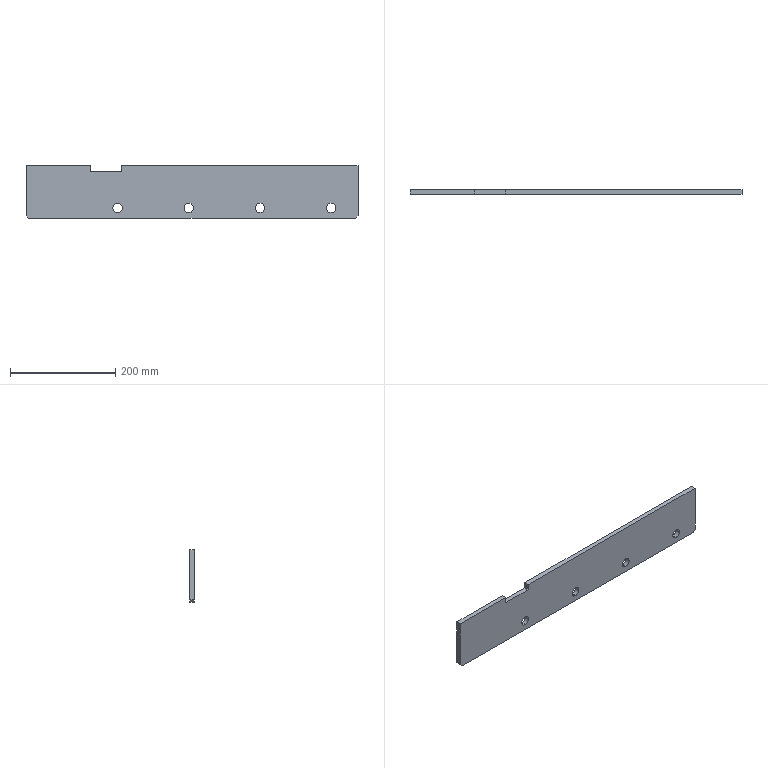Part | SolidWorks | features FlatPattern 1, SMBaseFlange 1, SheetMetal 1 | 1 solid | 20 faces | box 630 x 9 x 100 mm | volume 551134 mm3 | plane 12 | cylinder 8 | commonest cylinder face diameters 18 x8
STEP:
#1=CARTESIAN_POINT('',(579.,-9.,-89.));
#2=VERTEX_POINT('',#1);
#3=CARTESIAN_POINT('',(579.,-9.,-71.));
#4=VERTEX_POINT('',#3);
#5=CARTESIAN_POINT('',(579.,-9.,-80.));
#6=DIRECTION('',(0.,1.,0.));
#7=DIRECTION('',(0.,0.,1.));
#8=AXIS2_PLACEMENT_3D('',#5,#6,#7);
#9=CIRCLE('',#8,9.);
#10=EDGE_CURVE('',#2,#4,#9,.T.);
#11=ORIENTED_EDGE('',*,*,#10,.F.);
#12=CARTESIAN_POINT('',(579.,0.,-89.));
#13=VERTEX_POINT('',#12);
#14=CARTESIAN_POINT('',(579.,-9.,-89.));
#15=DIRECTION('',(0.,1.,0.));
#16=VECTOR('',#15,1000.);
#17=LINE('',#14,#16);
#18=EDGE_CURVE('',#2,#13,#17,.T.);
#19=ORIENTED_EDGE('',*,*,#18,.T.);
#20=CARTESIAN_POINT('',(579.,0.,-71.));
#21=VERTEX_POINT('',#20);
#22=CARTESIAN_POINT('',(579.,0.,-80.));
#23=DIRECTION('',(0.,1.,0.));
#24=DIRECTION('',(0.,0.,1.));
#25=AXIS2_PLACEMENT_3D('',#22,#23,#24);
#26=CIRCLE('',#25,9.);
#27=EDGE_CURVE('',#13,#21,#26,.T.);
#28=ORIENTED_EDGE('',*,*,#27,.T.);
#29=CARTESIAN_POINT('',(579.,-9.,-71.));
#30=DIRECTION('',(0.,1.,0.));
#31=VECTOR('',#30,1000.);
#32=LINE('',#29,#31);
#33=EDGE_CURVE('',#4,#21,#32,.T.);
#34=ORIENTED_EDGE('',*,*,#33,.F.);
#35=EDGE_LOOP('',(#11,#19,#28,#34));
#36=FACE_OUTER_BOUND('',#35,.T.);
#37=CARTESIAN_POINT('',(579.,-9.,-80.));
#38=DIRECTION('',(0.,1.,0.));
#39=DIRECTION('',(0.,0.,1.));
#40=AXIS2_PLACEMENT_3D('',#37,#38,#39);
#41=CYLINDRICAL_SURFACE('',#40,9.);
#42=ADVANCED_FACE('',(#36),#41,.F.);
#43=CARTESIAN_POINT('',(444.,-9.,-89.));
#44=VERTEX_POINT('',#43);
#45=CARTESIAN_POINT('',(444.,-9.,-71.));
#46=VERTEX_POINT('',#45);
#47=CARTESIAN_POINT('',(444.,-9.,-80.));
#48=DIRECTION('',(0.,1.,0.));
#49=DIRECTION('',(0.,0.,1.));
#50=AXIS2_PLACEMENT_3D('',#47,#48,#49);
#51=CIRCLE('',#50,9.);
#52=EDGE_CURVE('',#44,#46,#51,.T.);
#53=ORIENTED_EDGE('',*,*,#52,.F.);
#54=CARTESIAN_POINT('',(444.,0.,-89.));
#55=VERTEX_POINT('',#54);
#56=CARTESIAN_POINT('',(444.,-9.,-89.));
#57=DIRECTION('',(0.,1.,0.));
#58=VECTOR('',#57,1000.);
#59=LINE('',#56,#58);
#60=EDGE_CURVE('',#44,#55,#59,.T.);
#61=ORIENTED_EDGE('',*,*,#60,.T.);
#62=CARTESIAN_POINT('',(444.,0.,-71.));
#63=VERTEX_POINT('',#62);
#64=CARTESIAN_POINT('',(444.,0.,-80.));
#65=DIRECTION('',(0.,1.,0.));
#66=DIRECTION('',(0.,0.,1.));
#67=AXIS2_PLACEMENT_3D('',#64,#65,#66);
#68=CIRCLE('',#67,9.);
#69=EDGE_CURVE('',#55,#63,#68,.T.);
#70=ORIENTED_EDGE('',*,*,#69,.T.);
#71=CARTESIAN_POINT('',(444.,-9.,-71.));
#72=DIRECTION('',(0.,1.,0.));
#73=VECTOR('',#72,1000.);
#74=LINE('',#71,#73);
#75=EDGE_CURVE('',#46,#63,#74,.T.);
#76=ORIENTED_EDGE('',*,*,#75,.F.);
#77=EDGE_LOOP('',(#53,#61,#70,#76));
#78=FACE_OUTER_BOUND('',#77,.T.);
#79=CARTESIAN_POINT('',(444.,-9.,-80.));
#80=DIRECTION('',(0.,1.,0.));
#81=DIRECTION('',(0.,0.,1.));
#82=AXIS2_PLACEMENT_3D('',#79,#80,#81);
#83=CYLINDRICAL_SURFACE('',#82,9.);
#84=ADVANCED_FACE('',(#78),#83,.F.);
#85=CARTESIAN_POINT('',(309.,-9.,-89.));
#86=VERTEX_POINT('',#85);
#87=CARTESIAN_POINT('',(309.,-9.,-71.));
#88=VERTEX_POINT('',#87);
#89=CARTESIAN_POINT('',(309.,-9.,-80.));
#90=DIRECTION('',(0.,1.,0.));
#91=DIRECTION('',(0.,0.,1.));
#92=AXIS2_PLACEMENT_3D('',#89,#90,#91);
#93=CIRCLE('',#92,9.);
#94=EDGE_CURVE('',#86,#88,#93,.T.);
#95=ORIENTED_EDGE('',*,*,#94,.F.);
#96=CARTESIAN_POINT('',(309.,0.,-89.));
#97=VERTEX_POINT('',#96);
#98=CARTESIAN_POINT('',(309.,-9.,-89.));
#99=DIRECTION('',(0.,1.,0.));
#100=VECTOR('',#99,1000.);
#101=LINE('',#98,#100);
#102=EDGE_CURVE('',#86,#97,#101,.T.);
#103=ORIENTED_EDGE('',*,*,#102,.T.);
#104=CARTESIAN_POINT('',(309.,0.,-71.));
#105=VERTEX_POINT('',#104);
#106=CARTESIAN_POINT('',(309.,0.,-80.));
#107=DIRECTION('',(0.,1.,0.));
#108=DIRECTION('',(0.,0.,1.));
#109=AXIS2_PLACEMENT_3D('',#106,#107,#108);
#110=CIRCLE('',#109,9.);
#111=EDGE_CURVE('',#97,#105,#110,.T.);
#112=ORIENTED_EDGE('',*,*,#111,.T.);
#113=CARTESIAN_POINT('',(309.,-9.,-71.));
#114=DIRECTION('',(0.,1.,0.));
#115=VECTOR('',#114,1000.);
#116=LINE('',#113,#115);
#117=EDGE_CURVE('',#88,#105,#116,.T.);
#118=ORIENTED_EDGE('',*,*,#117,.F.);
#119=EDGE_LOOP('',(#95,#103,#112,#118));
#120=FACE_OUTER_BOUND('',#119,.T.);
#121=CARTESIAN_POINT('',(309.,-9.,-80.));
#122=DIRECTION('',(0.,1.,0.));
#123=DIRECTION('',(0.,0.,1.));
#124=AXIS2_PLACEMENT_3D('',#121,#122,#123);
#125=CYLINDRICAL_SURFACE('',#124,9.);
#126=ADVANCED_FACE('',(#120),#125,.F.);
#127=CARTESIAN_POINT('',(174.,-9.,-89.));
#128=VERTEX_POINT('',#127);
#129=CARTESIAN_POINT('',(174.,-9.,-71.));
#130=VERTEX_POINT('',#129);
#131=CARTESIAN_POINT('',(174.,-9.,-80.));
#132=DIRECTION('',(0.,1.,0.));
#133=DIRECTION('',(0.,0.,1.));
#134=AXIS2_PLACEMENT_3D('',#131,#132,#133);
#135=CIRCLE('',#134,9.);
#136=EDGE_CURVE('',#128,#130,#135,.T.);
#137=ORIENTED_EDGE('',*,*,#136,.F.);
#138=CARTESIAN_POINT('',(174.,0.,-89.));
#139=VERTEX_POINT('',#138);
#140=CARTESIAN_POINT('',(174.,-9.,-89.));
#141=DIRECTION('',(0.,1.,0.));
#142=VECTOR('',#141,1000.);
#143=LINE('',#140,#142);
#144=EDGE_CURVE('',#128,#139,#143,.T.);
#145=ORIENTED_EDGE('',*,*,#144,.T.);
#146=CARTESIAN_POINT('',(174.,0.,-71.));
#147=VERTEX_POINT('',#146);
#148=CARTESIAN_POINT('',(174.,0.,-80.));
#149=DIRECTION('',(0.,1.,0.));
#150=DIRECTION('',(0.,0.,1.));
#151=AXIS2_PLACEMENT_3D('',#148,#149,#150);
#152=CIRCLE('',#151,9.);
#153=EDGE_CURVE('',#139,#147,#152,.T.);
#154=ORIENTED_EDGE('',*,*,#153,.T.);
#155=CARTESIAN_POINT('',(174.,-9.,-71.));
#156=DIRECTION('',(0.,1.,0.));
#157=VECTOR('',#156,1000.);
#158=LINE('',#155,#157);
#159=EDGE_CURVE('',#130,#147,#158,.T.);
#160=ORIENTED_EDGE('',*,*,#159,.F.);
#161=EDGE_LOOP('',(#137,#145,#154,#160));
#162=FACE_OUTER_BOUND('',#161,.T.);
#163=CARTESIAN_POINT('',(174.,-9.,-80.));
#164=DIRECTION('',(0.,1.,0.));
#165=DIRECTION('',(0.,0.,1.));
#166=AXIS2_PLACEMENT_3D('',#163,#164,#165);
#167=CYLINDRICAL_SURFACE('',#166,9.);
#168=ADVANCED_FACE('',(#162),#167,.F.);
#169=CARTESIAN_POINT('',(0.,0.,-95.));
#170=VERTEX_POINT('',#169);
#171=CARTESIAN_POINT('',(0.,0.,0.));
#172=VERTEX_POINT('',#171);
#173=CARTESIAN_POINT('',(0.,0.,0.));
#174=DIRECTION('',(0.,0.,1.));
#175=VECTOR('',#174,1000.);
#176=LINE('',#173,#175);
#177=EDGE_CURVE('',#170,#172,#176,.T.);
#178=ORIENTED_EDGE('',*,*,#177,.F.);
#179=CARTESIAN_POINT('',(0.,-9.,-95.));
#180=VERTEX_POINT('',#179);
#181=CARTESIAN_POINT('',(0.,-9.,-95.));
#182=DIRECTION('',(0.,1.,0.));
#183=VECTOR('',#182,1000.);
#184=LINE('',#181,#183);
#185=EDGE_CURVE('',#180,#170,#184,.T.);
#186=ORIENTED_EDGE('',*,*,#185,.F.);
#187=CARTESIAN_POINT('',(0.,-9.,0.));
#188=VERTEX_POINT('',#187);
#189=CARTESIAN_POINT('',(0.,-9.,0.));
#190=DIRECTION('',(0.,0.,1.));
#191=VECTOR('',#190,1000.);
#192=LINE('',#189,#191);
#193=EDGE_CURVE('',#180,#188,#192,.T.);
#194=ORIENTED_EDGE('',*,*,#193,.T.);
#195=CARTESIAN_POINT('',(0.,-9.,0.));
#196=DIRECTION('',(0.,1.,0.));
#197=VECTOR('',#196,1000.);
#198=LINE('',#195,#197);
#199=EDGE_CURVE('',#188,#172,#198,.T.);
#200=ORIENTED_EDGE('',*,*,#199,.T.);
#201=EDGE_LOOP('',(#178,#186,#194,#200));
#202=FACE_OUTER_BOUND('',#201,.T.);
#203=CARTESIAN_POINT('',(0.,-9.,0.));
#204=DIRECTION('',(-1.,0.,0.));
#205=DIRECTION('',(0.,0.,1.));
#206=AXIS2_PLACEMENT_3D('',#203,#204,#205);
#207=PLANE('',#206);
#208=ADVANCED_FACE('',(#202),#207,.T.);
#209=CARTESIAN_POINT('',(5.,0.,-100.));
#210=VERTEX_POINT('',#209);
#211=CARTESIAN_POINT('',(0.,0.,-95.));
#212=DIRECTION('',(-0.7071,0.,0.7071));
#213=VECTOR('',#212,1000.);
#214=LINE('',#211,#213);
#215=EDGE_CURVE('',#210,#170,#214,.T.);
#216=ORIENTED_EDGE('',*,*,#215,.F.);
#217=CARTESIAN_POINT('',(5.,-9.,-100.));
#218=VERTEX_POINT('',#217);
#219=CARTESIAN_POINT('',(5.,-9.,-100.));
#220=DIRECTION('',(0.,1.,0.));
#221=VECTOR('',#220,1000.);
#222=LINE('',#219,#221);
#223=EDGE_CURVE('',#218,#210,#222,.T.);
#224=ORIENTED_EDGE('',*,*,#223,.F.);
#225=CARTESIAN_POINT('',(0.,-9.,-95.));
#226=DIRECTION('',(-0.7071,0.,0.7071));
#227=VECTOR('',#226,1000.);
#228=LINE('',#225,#227);
#229=EDGE_CURVE('',#218,#180,#228,.T.);
#230=ORIENTED_EDGE('',*,*,#229,.T.);
#231=ORIENTED_EDGE('',*,*,#185,.T.);
#232=EDGE_LOOP('',(#216,#224,#230,#231));
#233=FACE_OUTER_BOUND('',#232,.T.);
#234=CARTESIAN_POINT('',(0.,-9.,-95.));
#235=DIRECTION('',(-0.7071,0.,-0.7071));
#236=DIRECTION('',(-0.7071,0.,0.7071));
#237=AXIS2_PLACEMENT_3D('',#234,#235,#236);
#238=PLANE('',#237);
#239=ADVANCED_FACE('',(#233),#238,.T.);
#240=CARTESIAN_POINT('',(625.,0.,-100.));
#241=VERTEX_POINT('',#240);
#242=CARTESIAN_POINT('',(5.,0.,-100.));
#243=DIRECTION('',(-1.,0.,0.));
#244=VECTOR('',#243,1000.);
#245=LINE('',#242,#244);
#246=EDGE_CURVE('',#241,#210,#245,.T.);
#247=ORIENTED_EDGE('',*,*,#246,.F.);
#248=CARTESIAN_POINT('',(625.,-9.,-100.));
#249=VERTEX_POINT('',#248);
#250=CARTESIAN_POINT('',(625.,-9.,-100.));
#251=DIRECTION('',(0.,1.,0.));
#252=VECTOR('',#251,1000.);
#253=LINE('',#250,#252);
#254=EDGE_CURVE('',#249,#241,#253,.T.);
#255=ORIENTED_EDGE('',*,*,#254,.F.);
#256=CARTESIAN_POINT('',(5.,-9.,-100.));
#257=DIRECTION('',(-1.,0.,0.));
#258=VECTOR('',#257,1000.);
#259=LINE('',#256,#258);
#260=EDGE_CURVE('',#249,#218,#259,.T.);
#261=ORIENTED_EDGE('',*,*,#260,.T.);
#262=ORIENTED_EDGE('',*,*,#223,.T.);
#263=EDGE_LOOP('',(#247,#255,#261,#262));
#264=FACE_OUTER_BOUND('',#263,.T.);
#265=CARTESIAN_POINT('',(5.,-9.,-100.));
#266=DIRECTION('',(0.,0.,-1.));
#267=DIRECTION('',(-1.,0.,0.));
#268=AXIS2_PLACEMENT_3D('',#265,#266,#267);
#269=PLANE('',#268);
#270=ADVANCED_FACE('',(#264),#269,.T.);
#271=CARTESIAN_POINT('',(630.,0.,-95.));
#272=VERTEX_POINT('',#271);
#273=CARTESIAN_POINT('',(625.,0.,-100.));
#274=DIRECTION('',(-0.7071,0.,-0.7071));
#275=VECTOR('',#274,1000.);
#276=LINE('',#273,#275);
#277=EDGE_CURVE('',#272,#241,#276,.T.);
#278=ORIENTED_EDGE('',*,*,#277,.F.);
#279=CARTESIAN_POINT('',(630.,-9.,-95.));
#280=VERTEX_POINT('',#279);
#281=CARTESIAN_POINT('',(630.,-9.,-95.));
#282=DIRECTION('',(0.,1.,0.));
#283=VECTOR('',#282,1000.);
#284=LINE('',#281,#283);
#285=EDGE_CURVE('',#280,#272,#284,.T.);
#286=ORIENTED_EDGE('',*,*,#285,.F.);
#287=CARTESIAN_POINT('',(625.,-9.,-100.));
#288=DIRECTION('',(-0.7071,0.,-0.7071));
#289=VECTOR('',#288,1000.);
#290=LINE('',#287,#289);
#291=EDGE_CURVE('',#280,#249,#290,.T.);
#292=ORIENTED_EDGE('',*,*,#291,.T.);
#293=ORIENTED_EDGE('',*,*,#254,.T.);
#294=EDGE_LOOP('',(#278,#286,#292,#293));
#295=FACE_OUTER_BOUND('',#294,.T.);
#296=CARTESIAN_POINT('',(625.,-9.,-100.));
#297=DIRECTION('',(0.7071,0.,-0.7071));
#298=DIRECTION('',(-0.7071,0.,-0.7071));
#299=AXIS2_PLACEMENT_3D('',#296,#297,#298);
#300=PLANE('',#299);
#301=ADVANCED_FACE('',(#295),#300,.T.);
#302=CARTESIAN_POINT('',(630.,0.,0.));
#303=VERTEX_POINT('',#302);
#304=CARTESIAN_POINT('',(630.,0.,0.));
#305=DIRECTION('',(0.,0.,-1.));
#306=VECTOR('',#305,1000.);
#307=LINE('',#304,#306);
#308=EDGE_CURVE('',#303,#272,#307,.T.);
#309=ORIENTED_EDGE('',*,*,#308,.F.);
#310=CARTESIAN_POINT('',(630.,-9.,0.));
#311=VERTEX_POINT('',#310);
#312=CARTESIAN_POINT('',(630.,-9.,0.));
#313=DIRECTION('',(0.,1.,0.));
#314=VECTOR('',#313,1000.);
#315=LINE('',#312,#314);
#316=EDGE_CURVE('',#311,#303,#315,.T.);
#317=ORIENTED_EDGE('',*,*,#316,.F.);
#318=CARTESIAN_POINT('',(630.,-9.,0.));
#319=DIRECTION('',(0.,0.,-1.));
#320=VECTOR('',#319,1000.);
#321=LINE('',#318,#320);
#322=EDGE_CURVE('',#311,#280,#321,.T.);
#323=ORIENTED_EDGE('',*,*,#322,.T.);
#324=ORIENTED_EDGE('',*,*,#285,.T.);
#325=EDGE_LOOP('',(#309,#317,#323,#324));
#326=FACE_OUTER_BOUND('',#325,.T.);
#327=CARTESIAN_POINT('',(630.,-9.,0.));
#328=DIRECTION('',(1.,0.,0.));
#329=DIRECTION('',(0.,0.,-1.));
#330=AXIS2_PLACEMENT_3D('',#327,#328,#329);
#331=PLANE('',#330);
#332=ADVANCED_FACE('',(#326),#331,.T.);
#333=CARTESIAN_POINT('',(182.,0.,0.));
#334=VERTEX_POINT('',#333);
#335=CARTESIAN_POINT('',(182.,0.,0.));
#336=DIRECTION('',(1.,0.,0.));
#337=VECTOR('',#336,1000.);
#338=LINE('',#335,#337);
#339=EDGE_CURVE('',#334,#303,#338,.T.);
#340=ORIENTED_EDGE('',*,*,#339,.F.);
#341=CARTESIAN_POINT('',(182.,-9.,0.));
#342=VERTEX_POINT('',#341);
#343=CARTESIAN_POINT('',(182.,-9.,0.));
#344=DIRECTION('',(0.,1.,0.));
#345=VECTOR('',#344,1000.);
#346=LINE('',#343,#345);
#347=EDGE_CURVE('',#342,#334,#346,.T.);
#348=ORIENTED_EDGE('',*,*,#347,.F.);
#349=CARTESIAN_POINT('',(182.,-9.,0.));
#350=DIRECTION('',(1.,0.,0.));
#351=VECTOR('',#350,1000.);
#352=LINE('',#349,#351);
#353=EDGE_CURVE('',#342,#311,#352,.T.);
#354=ORIENTED_EDGE('',*,*,#353,.T.);
#355=ORIENTED_EDGE('',*,*,#316,.T.);
#356=EDGE_LOOP('',(#340,#348,#354,#355));
#357=FACE_OUTER_BOUND('',#356,.T.);
#358=CARTESIAN_POINT('',(182.,-9.,0.));
#359=DIRECTION('',(0.,0.,1.));
#360=DIRECTION('',(1.,0.,0.));
#361=AXIS2_PLACEMENT_3D('',#358,#359,#360);
#362=PLANE('',#361);
#363=ADVANCED_FACE('',(#357),#362,.T.);
#364=CARTESIAN_POINT('',(182.,0.,-12.));
#365=VERTEX_POINT('',#364);
#366=CARTESIAN_POINT('',(182.,0.,-12.));
#367=DIRECTION('',(0.,0.,1.));
#368=VECTOR('',#367,1000.);
#369=LINE('',#366,#368);
#370=EDGE_CURVE('',#365,#334,#369,.T.);
#371=ORIENTED_EDGE('',*,*,#370,.F.);
#372=CARTESIAN_POINT('',(182.,-9.,-12.));
#373=VERTEX_POINT('',#372);
#374=CARTESIAN_POINT('',(182.,-9.,-12.));
#375=DIRECTION('',(0.,1.,0.));
#376=VECTOR('',#375,1000.);
#377=LINE('',#374,#376);
#378=EDGE_CURVE('',#373,#365,#377,.T.);
#379=ORIENTED_EDGE('',*,*,#378,.F.);
#380=CARTESIAN_POINT('',(182.,-9.,-12.));
#381=DIRECTION('',(0.,0.,1.));
#382=VECTOR('',#381,1000.);
#383=LINE('',#380,#382);
#384=EDGE_CURVE('',#373,#342,#383,.T.);
#385=ORIENTED_EDGE('',*,*,#384,.T.);
#386=ORIENTED_EDGE('',*,*,#347,.T.);
#387=EDGE_LOOP('',(#371,#379,#385,#386));
#388=FACE_OUTER_BOUND('',#387,.T.);
#389=CARTESIAN_POINT('',(182.,-9.,-12.));
#390=DIRECTION('',(-1.,0.,0.));
#391=DIRECTION('',(0.,0.,1.));
#392=AXIS2_PLACEMENT_3D('',#389,#390,#391);
#393=PLANE('',#392);
#394=ADVANCED_FACE('',(#388),#393,.T.);
#395=CARTESIAN_POINT('',(122.,0.,-12.));
#396=VERTEX_POINT('',#395);
#397=CARTESIAN_POINT('',(122.,0.,-12.));
#398=DIRECTION('',(1.,0.,0.));
#399=VECTOR('',#398,1000.);
#400=LINE('',#397,#399);
#401=EDGE_CURVE('',#396,#365,#400,.T.);
#402=ORIENTED_EDGE('',*,*,#401,.F.);
#403=CARTESIAN_POINT('',(122.,-9.,-12.));
#404=VERTEX_POINT('',#403);
#405=CARTESIAN_POINT('',(122.,-9.,-12.));
#406=DIRECTION('',(0.,1.,0.));
#407=VECTOR('',#406,1000.);
#408=LINE('',#405,#407);
#409=EDGE_CURVE('',#404,#396,#408,.T.);
#410=ORIENTED_EDGE('',*,*,#409,.F.);
#411=CARTESIAN_POINT('',(122.,-9.,-12.));
#412=DIRECTION('',(1.,0.,0.));
#413=VECTOR('',#412,1000.);
#414=LINE('',#411,#413);
#415=EDGE_CURVE('',#404,#373,#414,.T.);
#416=ORIENTED_EDGE('',*,*,#415,.T.);
#417=ORIENTED_EDGE('',*,*,#378,.T.);
#418=EDGE_LOOP('',(#402,#410,#416,#417));
#419=FACE_OUTER_BOUND('',#418,.T.);
#420=CARTESIAN_POINT('',(122.,-9.,-12.));
#421=DIRECTION('',(0.,0.,1.));
#422=DIRECTION('',(1.,0.,0.));
#423=AXIS2_PLACEMENT_3D('',#420,#421,#422);
#424=PLANE('',#423);
#425=ADVANCED_FACE('',(#419),#424,.T.);
#426=CARTESIAN_POINT('',(122.,0.,0.));
#427=VERTEX_POINT('',#426);
#428=CARTESIAN_POINT('',(122.,0.,0.));
#429=DIRECTION('',(0.,0.,-1.));
#430=VECTOR('',#429,1000.);
#431=LINE('',#428,#430);
#432=EDGE_CURVE('',#427,#396,#431,.T.);
#433=ORIENTED_EDGE('',*,*,#432,.F.);
#434=CARTESIAN_POINT('',(122.,-9.,0.));
#435=VERTEX_POINT('',#434);
#436=CARTESIAN_POINT('',(122.,-9.,0.));
#437=DIRECTION('',(0.,1.,0.));
#438=VECTOR('',#437,1000.);
#439=LINE('',#436,#438);
#440=EDGE_CURVE('',#435,#427,#439,.T.);
#441=ORIENTED_EDGE('',*,*,#440,.F.);
#442=CARTESIAN_POINT('',(122.,-9.,0.));
#443=DIRECTION('',(0.,0.,-1.));
#444=VECTOR('',#443,1000.);
#445=LINE('',#442,#444);
#446=EDGE_CURVE('',#435,#404,#445,.T.);
#447=ORIENTED_EDGE('',*,*,#446,.T.);
#448=ORIENTED_EDGE('',*,*,#409,.T.);
#449=EDGE_LOOP('',(#433,#441,#447,#448));
#450=FACE_OUTER_BOUND('',#449,.T.);
#451=CARTESIAN_POINT('',(122.,-9.,0.));
#452=DIRECTION('',(1.,0.,0.));
#453=DIRECTION('',(0.,0.,-1.));
#454=AXIS2_PLACEMENT_3D('',#451,#452,#453);
#455=PLANE('',#454);
#456=ADVANCED_FACE('',(#450),#455,.T.);
#457=CARTESIAN_POINT('',(0.,0.,0.));
#458=DIRECTION('',(1.,0.,0.));
#459=VECTOR('',#458,1000.);
#460=LINE('',#457,#459);
#461=EDGE_CURVE('',#172,#427,#460,.T.);
#462=ORIENTED_EDGE('',*,*,#461,.F.);
#463=ORIENTED_EDGE('',*,*,#199,.F.);
#464=CARTESIAN_POINT('',(0.,-9.,0.));
#465=DIRECTION('',(1.,0.,0.));
#466=VECTOR('',#465,1000.);
#467=LINE('',#464,#466);
#468=EDGE_CURVE('',#188,#435,#467,.T.);
#469=ORIENTED_EDGE('',*,*,#468,.T.);
#470=ORIENTED_EDGE('',*,*,#440,.T.);
#471=EDGE_LOOP('',(#462,#463,#469,#470));
#472=FACE_OUTER_BOUND('',#471,.T.);
#473=CARTESIAN_POINT('',(0.,-9.,0.));
#474=DIRECTION('',(0.,0.,1.));
#475=DIRECTION('',(1.,0.,0.));
#476=AXIS2_PLACEMENT_3D('',#473,#474,#475);
#477=PLANE('',#476);
#478=ADVANCED_FACE('',(#472),#477,.T.);
#479=CARTESIAN_POINT('',(579.,-9.,-80.));
#480=DIRECTION('',(0.,1.,0.));
#481=DIRECTION('',(0.,0.,1.));
#482=AXIS2_PLACEMENT_3D('',#479,#480,#481);
#483=CIRCLE('',#482,9.);
#484=EDGE_CURVE('',#4,#2,#483,.T.);
#485=ORIENTED_EDGE('',*,*,#484,.T.);
#486=ORIENTED_EDGE('',*,*,#10,.T.);
#487=EDGE_LOOP('',(#485,#486));
#488=FACE_BOUND('',#487,.T.);
#489=CARTESIAN_POINT('',(444.,-9.,-80.));
#490=DIRECTION('',(0.,1.,0.));
#491=DIRECTION('',(0.,0.,1.));
#492=AXIS2_PLACEMENT_3D('',#489,#490,#491);
#493=CIRCLE('',#492,9.);
#494=EDGE_CURVE('',#46,#44,#493,.T.);
#495=ORIENTED_EDGE('',*,*,#494,.T.);
#496=ORIENTED_EDGE('',*,*,#52,.T.);
#497=EDGE_LOOP('',(#495,#496));
#498=FACE_BOUND('',#497,.T.);
#499=CARTESIAN_POINT('',(309.,-9.,-80.));
#500=DIRECTION('',(0.,1.,0.));
#501=DIRECTION('',(0.,0.,1.));
#502=AXIS2_PLACEMENT_3D('',#499,#500,#501);
#503=CIRCLE('',#502,9.);
#504=EDGE_CURVE('',#88,#86,#503,.T.);
#505=ORIENTED_EDGE('',*,*,#504,.T.);
#506=ORIENTED_EDGE('',*,*,#94,.T.);
#507=EDGE_LOOP('',(#505,#506));
#508=FACE_BOUND('',#507,.T.);
#509=CARTESIAN_POINT('',(174.,-9.,-80.));
#510=DIRECTION('',(0.,1.,0.));
#511=DIRECTION('',(0.,0.,1.));
#512=AXIS2_PLACEMENT_3D('',#509,#510,#511);
#513=CIRCLE('',#512,9.);
#514=EDGE_CURVE('',#130,#128,#513,.T.);
#515=ORIENTED_EDGE('',*,*,#514,.T.);
#516=ORIENTED_EDGE('',*,*,#136,.T.);
#517=EDGE_LOOP('',(#515,#516));
#518=FACE_BOUND('',#517,.T.);
#519=ORIENTED_EDGE('',*,*,#193,.F.);
#520=ORIENTED_EDGE('',*,*,#229,.F.);
#521=ORIENTED_EDGE('',*,*,#260,.F.);
#522=ORIENTED_EDGE('',*,*,#291,.F.);
#523=ORIENTED_EDGE('',*,*,#322,.F.);
#524=ORIENTED_EDGE('',*,*,#353,.F.);
#525=ORIENTED_EDGE('',*,*,#384,.F.);
#526=ORIENTED_EDGE('',*,*,#415,.F.);
#527=ORIENTED_EDGE('',*,*,#446,.F.);
#528=ORIENTED_EDGE('',*,*,#468,.F.);
#529=EDGE_LOOP('',(#519,#520,#521,#522,#523,#524,#525,#526,#527,#528));
#530=FACE_OUTER_BOUND('',#529,.T.);
#531=CARTESIAN_POINT('',(0.,-9.,0.));
#532=DIRECTION('',(0.,-1.,0.));
#533=DIRECTION('',(0.,0.,-1.));
#534=AXIS2_PLACEMENT_3D('',#531,#532,#533);
#535=PLANE('',#534);
#536=ADVANCED_FACE('',(#488,#498,#508,#518,#530),#535,.T.);
#537=CARTESIAN_POINT('',(579.,0.,-80.));
#538=DIRECTION('',(0.,1.,0.));
#539=DIRECTION('',(0.,0.,1.));
#540=AXIS2_PLACEMENT_3D('',#537,#538,#539);
#541=CIRCLE('',#540,9.);
#542=EDGE_CURVE('',#21,#13,#541,.T.);
#543=ORIENTED_EDGE('',*,*,#542,.F.);
#544=ORIENTED_EDGE('',*,*,#27,.F.);
#545=EDGE_LOOP('',(#543,#544));
#546=FACE_BOUND('',#545,.T.);
#547=CARTESIAN_POINT('',(444.,0.,-80.));
#548=DIRECTION('',(0.,1.,0.));
#549=DIRECTION('',(0.,0.,1.));
#550=AXIS2_PLACEMENT_3D('',#547,#548,#549);
#551=CIRCLE('',#550,9.);
#552=EDGE_CURVE('',#63,#55,#551,.T.);
#553=ORIENTED_EDGE('',*,*,#552,.F.);
#554=ORIENTED_EDGE('',*,*,#69,.F.);
#555=EDGE_LOOP('',(#553,#554));
#556=FACE_BOUND('',#555,.T.);
#557=CARTESIAN_POINT('',(309.,0.,-80.));
#558=DIRECTION('',(0.,1.,0.));
#559=DIRECTION('',(0.,0.,1.));
#560=AXIS2_PLACEMENT_3D('',#557,#558,#559);
#561=CIRCLE('',#560,9.);
#562=EDGE_CURVE('',#105,#97,#561,.T.);
#563=ORIENTED_EDGE('',*,*,#562,.F.);
#564=ORIENTED_EDGE('',*,*,#111,.F.);
#565=EDGE_LOOP('',(#563,#564));
#566=FACE_BOUND('',#565,.T.);
#567=CARTESIAN_POINT('',(174.,0.,-80.));
#568=DIRECTION('',(0.,1.,0.));
#569=DIRECTION('',(0.,0.,1.));
#570=AXIS2_PLACEMENT_3D('',#567,#568,#569);
#571=CIRCLE('',#570,9.);
#572=EDGE_CURVE('',#147,#139,#571,.T.);
#573=ORIENTED_EDGE('',*,*,#572,.F.);
#574=ORIENTED_EDGE('',*,*,#153,.F.);
#575=EDGE_LOOP('',(#573,#574));
#576=FACE_BOUND('',#575,.T.);
#577=ORIENTED_EDGE('',*,*,#177,.T.);
#578=ORIENTED_EDGE('',*,*,#461,.T.);
#579=ORIENTED_EDGE('',*,*,#432,.T.);
#580=ORIENTED_EDGE('',*,*,#401,.T.);
#581=ORIENTED_EDGE('',*,*,#370,.T.);
#582=ORIENTED_EDGE('',*,*,#339,.T.);
#583=ORIENTED_EDGE('',*,*,#308,.T.);
#584=ORIENTED_EDGE('',*,*,#277,.T.);
#585=ORIENTED_EDGE('',*,*,#246,.T.);
#586=ORIENTED_EDGE('',*,*,#215,.T.);
#587=EDGE_LOOP('',(#577,#578,#579,#580,#581,#582,#583,#584,#585,#586));
#588=FACE_OUTER_BOUND('',#587,.T.);
#589=CARTESIAN_POINT('',(0.,0.,0.));
#590=DIRECTION('',(0.,-1.,0.));
#591=DIRECTION('',(0.,0.,-1.));
#592=AXIS2_PLACEMENT_3D('',#589,#590,#591);
#593=PLANE('',#592);
#594=ADVANCED_FACE('',(#546,#556,#566,#576,#588),#593,.F.);
#595=ORIENTED_EDGE('',*,*,#144,.F.);
#596=ORIENTED_EDGE('',*,*,#514,.F.);
#597=ORIENTED_EDGE('',*,*,#159,.T.);
#598=ORIENTED_EDGE('',*,*,#572,.T.);
#599=EDGE_LOOP('',(#595,#596,#597,#598));
#600=FACE_OUTER_BOUND('',#599,.T.);
#601=CARTESIAN_POINT('',(174.,-9.,-80.));
#602=DIRECTION('',(0.,1.,0.));
#603=DIRECTION('',(0.,0.,1.));
#604=AXIS2_PLACEMENT_3D('',#601,#602,#603);
#605=CYLINDRICAL_SURFACE('',#604,9.);
#606=ADVANCED_FACE('',(#600),#605,.F.);
#607=ORIENTED_EDGE('',*,*,#102,.F.);
#608=ORIENTED_EDGE('',*,*,#504,.F.);
#609=ORIENTED_EDGE('',*,*,#117,.T.);
#610=ORIENTED_EDGE('',*,*,#562,.T.);
#611=EDGE_LOOP('',(#607,#608,#609,#610));
#612=FACE_OUTER_BOUND('',#611,.T.);
#613=CARTESIAN_POINT('',(309.,-9.,-80.));
#614=DIRECTION('',(0.,1.,0.));
#615=DIRECTION('',(0.,0.,1.));
#616=AXIS2_PLACEMENT_3D('',#613,#614,#615);
#617=CYLINDRICAL_SURFACE('',#616,9.);
#618=ADVANCED_FACE('',(#612),#617,.F.);
#619=ORIENTED_EDGE('',*,*,#60,.F.);
#620=ORIENTED_EDGE('',*,*,#494,.F.);
#621=ORIENTED_EDGE('',*,*,#75,.T.);
#622=ORIENTED_EDGE('',*,*,#552,.T.);
#623=EDGE_LOOP('',(#619,#620,#621,#622));
#624=FACE_OUTER_BOUND('',#623,.T.);
#625=CARTESIAN_POINT('',(444.,-9.,-80.));
#626=DIRECTION('',(0.,1.,0.));
#627=DIRECTION('',(0.,0.,1.));
#628=AXIS2_PLACEMENT_3D('',#625,#626,#627);
#629=CYLINDRICAL_SURFACE('',#628,9.);
#630=ADVANCED_FACE('',(#624),#629,.F.);
#631=ORIENTED_EDGE('',*,*,#18,.F.);
#632=ORIENTED_EDGE('',*,*,#484,.F.);
#633=ORIENTED_EDGE('',*,*,#33,.T.);
#634=ORIENTED_EDGE('',*,*,#542,.T.);
#635=EDGE_LOOP('',(#631,#632,#633,#634));
#636=FACE_OUTER_BOUND('',#635,.T.);
#637=CARTESIAN_POINT('',(579.,-9.,-80.));
#638=DIRECTION('',(0.,1.,0.));
#639=DIRECTION('',(0.,0.,1.));
#640=AXIS2_PLACEMENT_3D('',#637,#638,#639);
#641=CYLINDRICAL_SURFACE('',#640,9.);
#642=ADVANCED_FACE('',(#636),#641,.F.);
#643=CLOSED_SHELL('',(#42,#84,#126,#168,#208,#239,#270,#301,#332,#363,#394,#425,#456,#478,#536,#594,#606,#618,#630,#642));
#644=MANIFOLD_SOLID_BREP('',#643);
#645=CARTESIAN_POINT('',(0.,0.,0.));
#646=DIRECTION('',(0.,0.,1.));
#647=DIRECTION('',(1.,0.,0.));
#648=AXIS2_PLACEMENT_3D('',#645,#646,#647);
#649=(LENGTH_UNIT()NAMED_UNIT(*)SI_UNIT(.MILLI.,.METRE.));
#650=UNCERTAINTY_MEASURE_WITH_UNIT(LENGTH_MEASURE(0.00001),#649,'','');
#651=(NAMED_UNIT(*)PLANE_ANGLE_UNIT()SI_UNIT($,.RADIAN.));
#652=(NAMED_UNIT(*)SI_UNIT($,.STERADIAN.)SOLID_ANGLE_UNIT());
#653=(GEOMETRIC_REPRESENTATION_CONTEXT(3)GLOBAL_UNCERTAINTY_ASSIGNED_CONTEXT((#650))GLOBAL_UNIT_ASSIGNED_CONTEXT((#649,#651,#652))REPRESENTATION_CONTEXT('',''));
#654=ADVANCED_BREP_SHAPE_REPRESENTATION('',(#644,#648),#653);